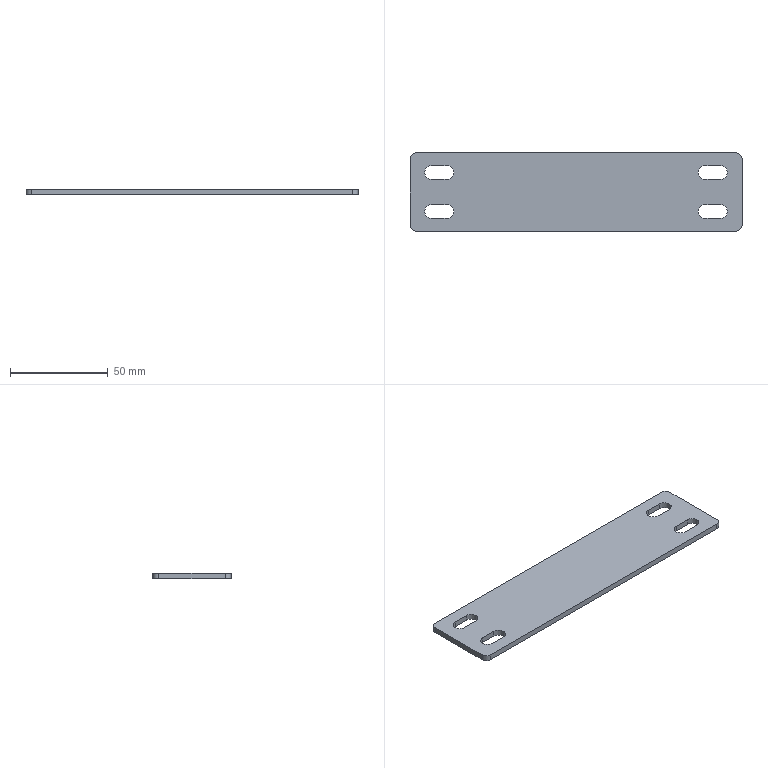Part | STEP file | PN_0006 guardrail connecting plate 210_Default<As Machined> | 1 solid | 26 faces | box 170 x 40 x 3 mm | volume 19243 mm3 | plane 14 | cylinder 12 | commonest cylinder face diameters 7 x8 6 x4